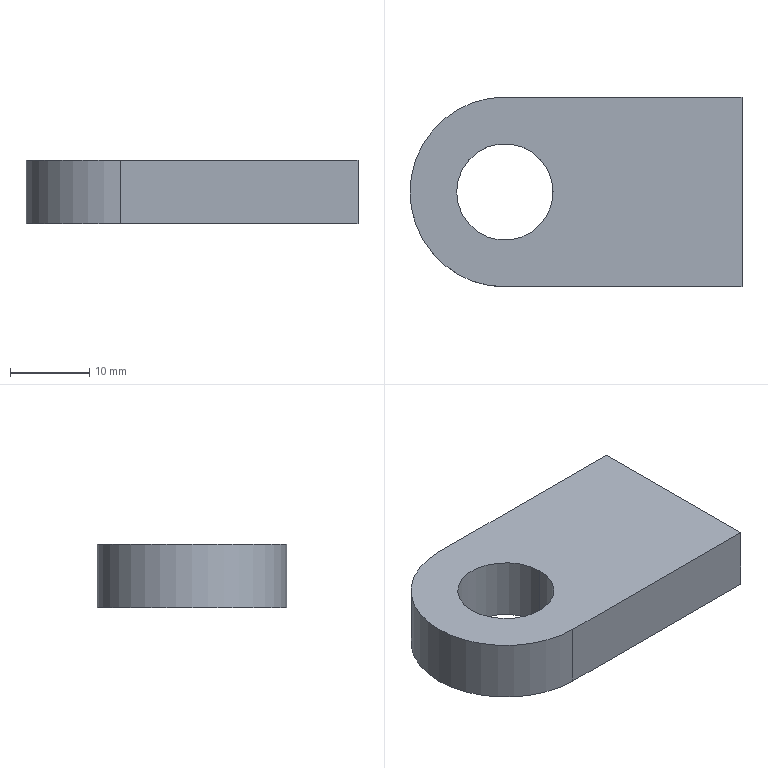Part | SolidWorks | features Extrusion 1 | 1 solid | 8 faces | box 42 x 24 x 8 mm | volume 6634 mm3 | plane 5 | cylinder 3 | commonest cylinder face diameters 12.2 x2 24 x1
STEP:
#1=CARTESIAN_POINT('',(-6.1,0.,-4.));
#2=VERTEX_POINT('',#1);
#3=CARTESIAN_POINT('',(6.1,0.,-4.));
#4=VERTEX_POINT('',#3);
#5=CARTESIAN_POINT('',(0.,0.,-4.));
#6=DIRECTION('',(0.,0.,1.));
#7=DIRECTION('',(1.,0.,0.));
#8=AXIS2_PLACEMENT_3D('',#5,#6,#7);
#9=CIRCLE('',#8,6.1);
#10=EDGE_CURVE('',#2,#4,#9,.T.);
#11=ORIENTED_EDGE('',*,*,#10,.F.);
#12=CARTESIAN_POINT('',(-6.1,0.,4.));
#13=VERTEX_POINT('',#12);
#14=CARTESIAN_POINT('',(-6.1,0.,-4.));
#15=DIRECTION('',(0.,0.,1.));
#16=VECTOR('',#15,1000.);
#17=LINE('',#14,#16);
#18=EDGE_CURVE('',#2,#13,#17,.T.);
#19=ORIENTED_EDGE('',*,*,#18,.T.);
#20=CARTESIAN_POINT('',(6.1,0.,4.));
#21=VERTEX_POINT('',#20);
#22=CARTESIAN_POINT('',(0.,0.,4.));
#23=DIRECTION('',(0.,0.,1.));
#24=DIRECTION('',(1.,0.,0.));
#25=AXIS2_PLACEMENT_3D('',#22,#23,#24);
#26=CIRCLE('',#25,6.1);
#27=EDGE_CURVE('',#13,#21,#26,.T.);
#28=ORIENTED_EDGE('',*,*,#27,.T.);
#29=CARTESIAN_POINT('',(6.1,0.,-4.));
#30=DIRECTION('',(0.,0.,1.));
#31=VECTOR('',#30,1000.);
#32=LINE('',#29,#31);
#33=EDGE_CURVE('',#4,#21,#32,.T.);
#34=ORIENTED_EDGE('',*,*,#33,.F.);
#35=EDGE_LOOP('',(#11,#19,#28,#34));
#36=FACE_OUTER_BOUND('',#35,.T.);
#37=CARTESIAN_POINT('',(0.,0.,-4.));
#38=DIRECTION('',(0.,0.,1.));
#39=DIRECTION('',(1.,0.,0.));
#40=AXIS2_PLACEMENT_3D('',#37,#38,#39);
#41=CYLINDRICAL_SURFACE('',#40,6.1);
#42=ADVANCED_FACE('',(#36),#41,.F.);
#43=CARTESIAN_POINT('',(0.,12.,4.));
#44=VERTEX_POINT('',#43);
#45=CARTESIAN_POINT('',(0.,-12.,4.));
#46=VERTEX_POINT('',#45);
#47=CARTESIAN_POINT('',(0.,0.,4.));
#48=DIRECTION('',(0.,0.,1.));
#49=DIRECTION('',(-1.,0.,0.));
#50=AXIS2_PLACEMENT_3D('',#47,#48,#49);
#51=CIRCLE('',#50,12.);
#52=EDGE_CURVE('',#44,#46,#51,.T.);
#53=ORIENTED_EDGE('',*,*,#52,.F.);
#54=CARTESIAN_POINT('',(0.,12.,-4.));
#55=VERTEX_POINT('',#54);
#56=CARTESIAN_POINT('',(0.,12.,-4.));
#57=DIRECTION('',(0.,0.,1.));
#58=VECTOR('',#57,1000.);
#59=LINE('',#56,#58);
#60=EDGE_CURVE('',#55,#44,#59,.T.);
#61=ORIENTED_EDGE('',*,*,#60,.F.);
#62=CARTESIAN_POINT('',(0.,-12.,-4.));
#63=VERTEX_POINT('',#62);
#64=CARTESIAN_POINT('',(0.,0.,-4.));
#65=DIRECTION('',(0.,0.,1.));
#66=DIRECTION('',(-1.,0.,0.));
#67=AXIS2_PLACEMENT_3D('',#64,#65,#66);
#68=CIRCLE('',#67,12.);
#69=EDGE_CURVE('',#55,#63,#68,.T.);
#70=ORIENTED_EDGE('',*,*,#69,.T.);
#71=CARTESIAN_POINT('',(0.,-12.,-4.));
#72=DIRECTION('',(0.,0.,1.));
#73=VECTOR('',#72,1000.);
#74=LINE('',#71,#73);
#75=EDGE_CURVE('',#63,#46,#74,.T.);
#76=ORIENTED_EDGE('',*,*,#75,.T.);
#77=EDGE_LOOP('',(#53,#61,#70,#76));
#78=FACE_OUTER_BOUND('',#77,.T.);
#79=CARTESIAN_POINT('',(0.,0.,-4.));
#80=DIRECTION('',(0.,0.,1.));
#81=DIRECTION('',(1.,0.,0.));
#82=AXIS2_PLACEMENT_3D('',#79,#80,#81);
#83=CYLINDRICAL_SURFACE('',#82,12.);
#84=ADVANCED_FACE('',(#78),#83,.T.);
#85=CARTESIAN_POINT('',(30.,12.,4.));
#86=VERTEX_POINT('',#85);
#87=CARTESIAN_POINT('',(0.,12.,4.));
#88=DIRECTION('',(-1.,0.,0.));
#89=VECTOR('',#88,1000.);
#90=LINE('',#87,#89);
#91=EDGE_CURVE('',#86,#44,#90,.T.);
#92=ORIENTED_EDGE('',*,*,#91,.F.);
#93=CARTESIAN_POINT('',(30.,12.,-4.));
#94=VERTEX_POINT('',#93);
#95=CARTESIAN_POINT('',(30.,12.,-4.));
#96=DIRECTION('',(0.,0.,1.));
#97=VECTOR('',#96,1000.);
#98=LINE('',#95,#97);
#99=EDGE_CURVE('',#94,#86,#98,.T.);
#100=ORIENTED_EDGE('',*,*,#99,.F.);
#101=CARTESIAN_POINT('',(0.,12.,-4.));
#102=DIRECTION('',(-1.,0.,0.));
#103=VECTOR('',#102,1000.);
#104=LINE('',#101,#103);
#105=EDGE_CURVE('',#94,#55,#104,.T.);
#106=ORIENTED_EDGE('',*,*,#105,.T.);
#107=ORIENTED_EDGE('',*,*,#60,.T.);
#108=EDGE_LOOP('',(#92,#100,#106,#107));
#109=FACE_OUTER_BOUND('',#108,.T.);
#110=CARTESIAN_POINT('',(0.,12.,-4.));
#111=DIRECTION('',(0.,1.,0.));
#112=DIRECTION('',(0.,0.,1.));
#113=AXIS2_PLACEMENT_3D('',#110,#111,#112);
#114=PLANE('',#113);
#115=ADVANCED_FACE('',(#109),#114,.T.);
#116=CARTESIAN_POINT('',(30.,-12.,4.));
#117=VERTEX_POINT('',#116);
#118=CARTESIAN_POINT('',(30.,12.,4.));
#119=DIRECTION('',(0.,1.,0.));
#120=VECTOR('',#119,1000.);
#121=LINE('',#118,#120);
#122=EDGE_CURVE('',#117,#86,#121,.T.);
#123=ORIENTED_EDGE('',*,*,#122,.F.);
#124=CARTESIAN_POINT('',(30.,-12.,-4.));
#125=VERTEX_POINT('',#124);
#126=CARTESIAN_POINT('',(30.,-12.,-4.));
#127=DIRECTION('',(0.,0.,1.));
#128=VECTOR('',#127,1000.);
#129=LINE('',#126,#128);
#130=EDGE_CURVE('',#125,#117,#129,.T.);
#131=ORIENTED_EDGE('',*,*,#130,.F.);
#132=CARTESIAN_POINT('',(30.,12.,-4.));
#133=DIRECTION('',(0.,1.,0.));
#134=VECTOR('',#133,1000.);
#135=LINE('',#132,#134);
#136=EDGE_CURVE('',#125,#94,#135,.T.);
#137=ORIENTED_EDGE('',*,*,#136,.T.);
#138=ORIENTED_EDGE('',*,*,#99,.T.);
#139=EDGE_LOOP('',(#123,#131,#137,#138));
#140=FACE_OUTER_BOUND('',#139,.T.);
#141=CARTESIAN_POINT('',(30.,12.,-4.));
#142=DIRECTION('',(1.,0.,0.));
#143=DIRECTION('',(0.,0.,-1.));
#144=AXIS2_PLACEMENT_3D('',#141,#142,#143);
#145=PLANE('',#144);
#146=ADVANCED_FACE('',(#140),#145,.T.);
#147=CARTESIAN_POINT('',(30.,-12.,4.));
#148=DIRECTION('',(1.,0.,0.));
#149=VECTOR('',#148,1000.);
#150=LINE('',#147,#149);
#151=EDGE_CURVE('',#46,#117,#150,.T.);
#152=ORIENTED_EDGE('',*,*,#151,.F.);
#153=ORIENTED_EDGE('',*,*,#75,.F.);
#154=CARTESIAN_POINT('',(30.,-12.,-4.));
#155=DIRECTION('',(1.,0.,0.));
#156=VECTOR('',#155,1000.);
#157=LINE('',#154,#156);
#158=EDGE_CURVE('',#63,#125,#157,.T.);
#159=ORIENTED_EDGE('',*,*,#158,.T.);
#160=ORIENTED_EDGE('',*,*,#130,.T.);
#161=EDGE_LOOP('',(#152,#153,#159,#160));
#162=FACE_OUTER_BOUND('',#161,.T.);
#163=CARTESIAN_POINT('',(30.,-12.,-4.));
#164=DIRECTION('',(0.,-1.,0.));
#165=DIRECTION('',(0.,0.,-1.));
#166=AXIS2_PLACEMENT_3D('',#163,#164,#165);
#167=PLANE('',#166);
#168=ADVANCED_FACE('',(#162),#167,.T.);
#169=CARTESIAN_POINT('',(0.,0.,-4.));
#170=DIRECTION('',(0.,0.,1.));
#171=DIRECTION('',(1.,0.,0.));
#172=AXIS2_PLACEMENT_3D('',#169,#170,#171);
#173=CIRCLE('',#172,6.1);
#174=EDGE_CURVE('',#4,#2,#173,.T.);
#175=ORIENTED_EDGE('',*,*,#174,.T.);
#176=ORIENTED_EDGE('',*,*,#10,.T.);
#177=EDGE_LOOP('',(#175,#176));
#178=FACE_BOUND('',#177,.T.);
#179=ORIENTED_EDGE('',*,*,#69,.F.);
#180=ORIENTED_EDGE('',*,*,#105,.F.);
#181=ORIENTED_EDGE('',*,*,#136,.F.);
#182=ORIENTED_EDGE('',*,*,#158,.F.);
#183=EDGE_LOOP('',(#179,#180,#181,#182));
#184=FACE_OUTER_BOUND('',#183,.T.);
#185=CARTESIAN_POINT('',(0.,0.,-4.));
#186=DIRECTION('',(0.,0.,-1.));
#187=DIRECTION('',(-1.,0.,0.));
#188=AXIS2_PLACEMENT_3D('',#185,#186,#187);
#189=PLANE('',#188);
#190=ADVANCED_FACE('',(#178,#184),#189,.T.);
#191=CARTESIAN_POINT('',(0.,0.,4.));
#192=DIRECTION('',(0.,0.,1.));
#193=DIRECTION('',(1.,0.,0.));
#194=AXIS2_PLACEMENT_3D('',#191,#192,#193);
#195=CIRCLE('',#194,6.1);
#196=EDGE_CURVE('',#21,#13,#195,.T.);
#197=ORIENTED_EDGE('',*,*,#196,.F.);
#198=ORIENTED_EDGE('',*,*,#27,.F.);
#199=EDGE_LOOP('',(#197,#198));
#200=FACE_BOUND('',#199,.T.);
#201=ORIENTED_EDGE('',*,*,#52,.T.);
#202=ORIENTED_EDGE('',*,*,#151,.T.);
#203=ORIENTED_EDGE('',*,*,#122,.T.);
#204=ORIENTED_EDGE('',*,*,#91,.T.);
#205=EDGE_LOOP('',(#201,#202,#203,#204));
#206=FACE_OUTER_BOUND('',#205,.T.);
#207=CARTESIAN_POINT('',(0.,0.,4.));
#208=DIRECTION('',(0.,0.,-1.));
#209=DIRECTION('',(-1.,0.,0.));
#210=AXIS2_PLACEMENT_3D('',#207,#208,#209);
#211=PLANE('',#210);
#212=ADVANCED_FACE('',(#200,#206),#211,.F.);
#213=ORIENTED_EDGE('',*,*,#18,.F.);
#214=ORIENTED_EDGE('',*,*,#174,.F.);
#215=ORIENTED_EDGE('',*,*,#33,.T.);
#216=ORIENTED_EDGE('',*,*,#196,.T.);
#217=EDGE_LOOP('',(#213,#214,#215,#216));
#218=FACE_OUTER_BOUND('',#217,.T.);
#219=CARTESIAN_POINT('',(0.,0.,-4.));
#220=DIRECTION('',(0.,0.,1.));
#221=DIRECTION('',(1.,0.,0.));
#222=AXIS2_PLACEMENT_3D('',#219,#220,#221);
#223=CYLINDRICAL_SURFACE('',#222,6.1);
#224=ADVANCED_FACE('',(#218),#223,.F.);
#225=CLOSED_SHELL('',(#42,#84,#115,#146,#168,#190,#212,#224));
#226=MANIFOLD_SOLID_BREP('',#225);
#227=CARTESIAN_POINT('',(0.,0.,0.));
#228=DIRECTION('',(0.,0.,1.));
#229=DIRECTION('',(1.,0.,0.));
#230=AXIS2_PLACEMENT_3D('',#227,#228,#229);
#231=(LENGTH_UNIT()NAMED_UNIT(*)SI_UNIT(.MILLI.,.METRE.));
#232=UNCERTAINTY_MEASURE_WITH_UNIT(LENGTH_MEASURE(0.00001),#231,'','');
#233=(NAMED_UNIT(*)PLANE_ANGLE_UNIT()SI_UNIT($,.RADIAN.));
#234=(NAMED_UNIT(*)SI_UNIT($,.STERADIAN.)SOLID_ANGLE_UNIT());
#235=(GEOMETRIC_REPRESENTATION_CONTEXT(3)GLOBAL_UNCERTAINTY_ASSIGNED_CONTEXT((#232))GLOBAL_UNIT_ASSIGNED_CONTEXT((#231,#233,#234))REPRESENTATION_CONTEXT('',''));
#236=ADVANCED_BREP_SHAPE_REPRESENTATION('',(#226,#230),#235);